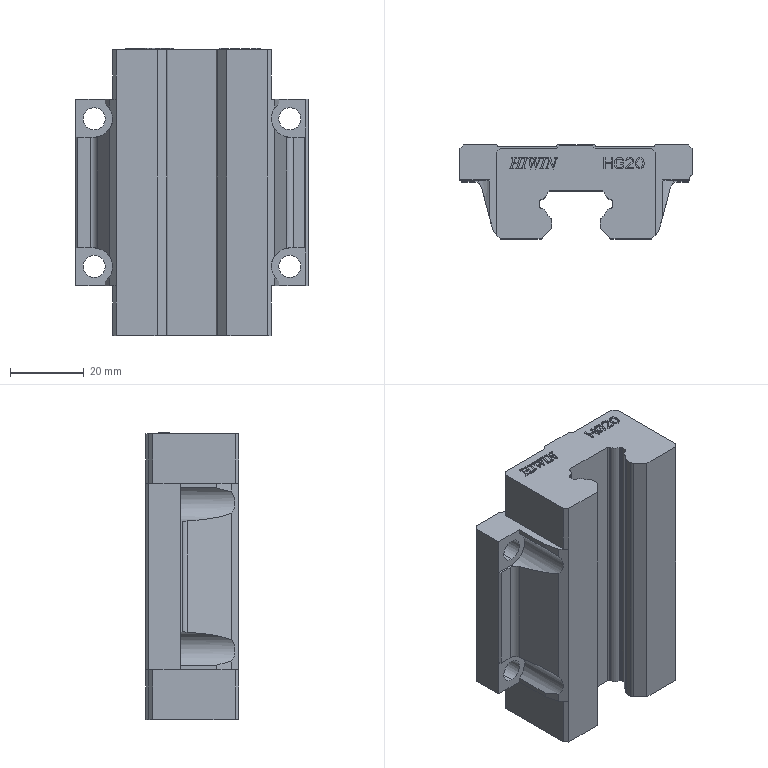Part | SolidWorks | features BaseBody 1 | 1 solid | 389 faces | box 63 x 25.4 x 77.8 mm | volume 78146 mm3 | plane 291 | spline 60 | cylinder 38 | commonest cylinder face diameters 1 x12 2 x8 6 x8 4.06 x4 10 x4 4 x2